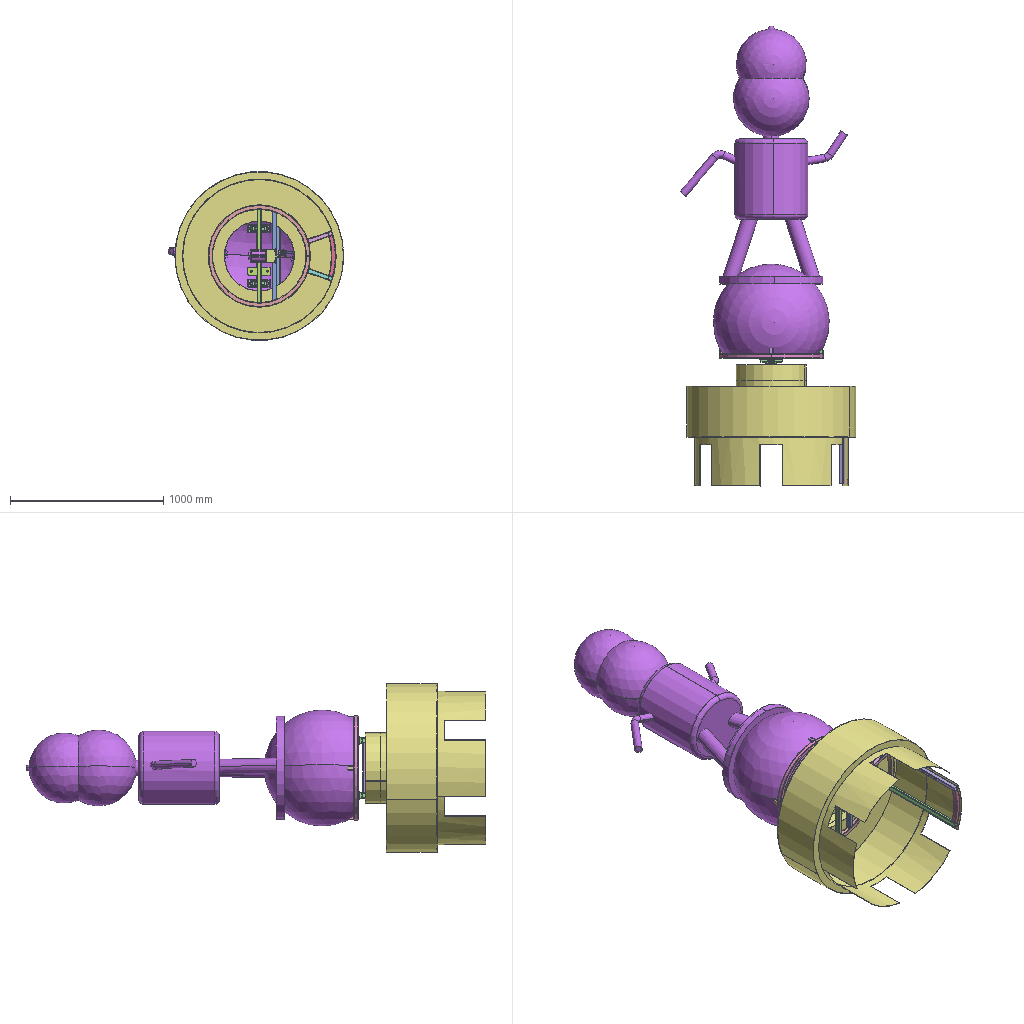Assembly | SolidWorks | 16 different items | 26 placed | box 1147 x 3005 x 1100 mm
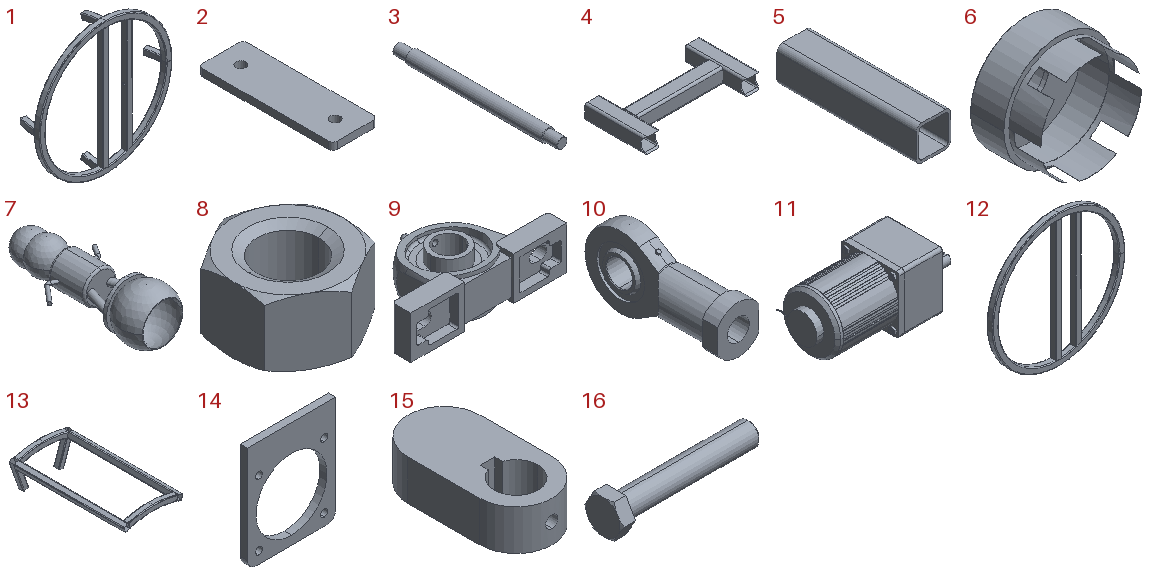Parts list (item | quantity | size | volume | features):
1 | x1 | 680 x 115 x 680 mm | 760065 mm3 | features ICE 3, WeldMemberFeat 2, CirPattern 1, WeldmentFeature 1
2 | x4 | 50 x 150 x 8 mm | 58308 mm3 | features Extrusion 1, HoleWzd 1
3 | x1 | 32 x 400 x 32 mm | 299686 mm3 | features Chamfer 1, Revolution 1
4 | x1 | 230 x 120 x 30 mm | 85383 mm3 | features ICE 1, WeldMemberFeat 1, WeldmentFeature 1
5 | x1 | 25 x 100 x 25 mm | 17370 mm3 | features WeldMemberFeat 1, WeldmentFeature 1
6 | x1 | 1104 x 790 x 1104 mm | 5979369 mm3 | features ICE 2, CirPattern 1, Revolution 1, Shell 1, WeldmentFeature 1
7 | x1 | 1093 x 2171 x 758 mm | 26788411 mm3 | features Sweep 4, ICE 3, Revolution 2, CombineBodies 1, Fillet 1, Shell 1
8 | x5 | 18 x 20.785 x 10.8 mm | 2109 mm3 | features ICE 2, RevCut 2, Extrusion 1
9 | x2 | 142 x 78.36 x 39.3 mm | 118845 mm3 | features Revolution 5, Cut 3, Boss 2, CirPattern 2, ICE 2, RevCut 2, Extrusion 1, RefAxis 1, SweepCut 1
10 | x1 | 19 x 67 x 34 mm | 14399 mm3 | features Revolution 3, ICE 2, RevCut 1
11 | x1 | 209 x 90.466 x 90 mm | 815406 mm3 | features ICE 12, Fillet 4, CirPattern 3, Chamfer 2, Revolution 2, Sweep 1
12 | x1 | 670 x 30 x 670 mm | 682937 mm3 | features ICE 1, WeldMemberFeat 1, WeldmentFeature 1
13 | x1 | 330 x 635 x 183.766 mm | 442860 mm3 | features 3DProfileFeature 1, WeldCornerFeat 1, WeldMemberFeat 1, WeldmentFeature 1
14 | x1 | 100 x 8 x 120 mm | 53836 mm3 | features CirPattern 1, Extrusion 1, Fillet 1, HoleWzd 1, ICE 1
15 | x1 | 25 x 50 x 14 mm | 12843 mm3 | features Extrusion 1, HoleWzd 1
16 | x3 | 77.5 x 20.785 x 18 mm | 9981 mm3 | features Chamfer 2, RevCut 2, Revolution 2, Extrusion 1, ICE 1
Mates (type | each side: item.copy, entity, surface, feature):
Width | 5.1 face plane Gb/t 6728—2002 Square hollow section steel 25×2-example.com(1) | 5.1 face plane Gb/t 6728—2002 Square hollow section steel 25×2-example.com(1) | 16.1 face plane Boss-Extrude1 | 16.1 face plane Boss-Extrude1
Concentric | 16.1 face cylinder Revolve1 | 8.1 face cylinder Boss-Extrude1
Coincident | 16.1 face plane Boss-Extrude1 | 8.1 face plane Boss-Extrude1
Concentric | 16.1 face cylinder Revolve1 | 10.1 face cylinder Cut-Revolve1
Parallel | 16.1 face plane Boss-Extrude1 | 10.1 face plane Cut-Extrude1
DistanceDim | 16.1 face plane Revolve1 | 10.1 face plane Revolve1
Coincident | 8.1 face plane Boss-Extrude1 | 10.1 face plane Revolve1
Coincident | 1.1 face plane Gb/t 6728—2002 Square hollow section steel 30×2-example.com(1) | 2.1 face plane Boss-Extrude1
DistanceDim | 16.2 face cylinder Revolve1 | 1.1 face plane Gb/t 6728—2002 Square hollow section steel 30×2-example.com(1)
Coincident | 1.1 face plane Gb/t 6728—2002 Square hollow section steel 30×2-example.com(1) | 16.2 face plane Boss-Extrude1
Coincident | 1.1 face plane Gb/t 6728—2002 Square hollow section steel 30×2-example.com(1) | 8.2 face plane Boss-Extrude1
Coincident | 2.1 face plane Boss-Extrude1 | 2.2 face plane Boss-Extrude1 | 2 times
Coincident | 2.1 face plane Boss-Extrude1 | 9.1 face plane Boss-Extrude1
Slot | 2.1 face cylinder Ø11.0 (11) Diameter Hole5 | 9.1 face cylinder Cut-Extrude3
Parallel | 2.1 face plane Boss-Extrude1 | 9.1 face plane Boss-Extrude1
DistanceDim | 2.2 face cylinder Ø11.0 (11) Diameter Hole5 | 2.1 face cylinder Ø11.0 (11) Diameter Hole5
Coincident | 2.2 face plane Boss-Extrude1 | 9.2 face plane Boss-Extrude1
Slot | 2.2 face cylinder Ø11.0 (11) Diameter Hole5 | 9.2 face cylinder Cut-Extrude3
Coincident | 2.3 face plane Boss-Extrude1 | 2.4 face plane Boss-Extrude1 | 3 times
Coincident | 4.1 face plane Gb/t 6728—2002 Square hollow section steel 30×2-example.com(1) | 2.3 face plane Boss-Extrude1
DistanceDim | 4.1 face plane Gb/t 6728—2002 Square hollow section steel 30×2-example.com(1) | 2.3 face plane Boss-Extrude1
Concentric | 3.1 face cylinder Revolve1 | 9.1 face cylinder Boss-Revolve5
Coincident | 3.1 face plane Revolve1 | 9.1 face plane Boss-Revolve5
Concentric | 3.1 face cylinder Revolve1 | 4.1 face cylinder Cut-Extrude1
Coincident | 9.1 face plane Boss-Extrude1 | 9.2 face plane Boss-Extrude1
Concentric | 8.2 face cylinder Boss-Extrude1 | 16.2 face cylinder Revolve1
DistanceDim | 8.3 face plane Boss-Extrude1 | 8.2 face plane Boss-Extrude1
Concentric | 16.2 face cylinder Revolve1 | 8.3 face cylinder Boss-Extrude1
Coincident | 1.1 face plane Gb/t 6728—2002 Square hollow section steel 30×2-example.com(1) | 7.1 face plane Revolve1
Concentric | 1.1 face cylinder Gb/t 6728—2002 Square hollow section steel 30×2-example.com(1) | 7.1 face cylinder Boss-Extrude2
Coincident | 11.1 face plane Boss-Extrude2 | 14.1 face plane Boss-Extrude1
Concentric | 11.1 face cylinder Cut-Extrude1 | 14.1 face cylinder Cut-Extrude1
Concentric | 11.1 face cylinder CirPattern3 | 14.1 face cylinder CirPattern1
Concentric | 11.1 face cylinder Revolve2 | 15.1 face cylinder Boss-Extrude1
Coincident | 11.1 face plane Revolve2 | 15.1 face plane Boss-Extrude1
Concentric | 15.1 face cylinder Boss-Extrude1 | 16.3 face cylinder Revolve1
Coincident | 15.1 face plane Boss-Extrude1 | 16.3 face plane Boss-Extrude1
Concentric | 16.3 face cylinder Revolve1 | 8.4 face cylinder Boss-Extrude1
Concentric | 16.3 face cylinder Revolve1 | 8.5 face cylinder Boss-Extrude1
Coincident | 8.4 face plane Boss-Extrude1 | 8.5 face plane Boss-Extrude1
Concentric | 16.3 face cylinder Revolve1 | 10.1 face cylinder Revolve2
Coincident | 8.4 face plane Boss-Extrude1 | 10.1 face plane Revolve2
Concentric | 12.1 face cylinder Gb/t 6728—2002 Square hollow section steel 30×2-example.com(1) | 13.1 face cylinder Gb/t 6728—2002 Square hollow section steel 30×2-example.com(1)
Coincident | 12.1 face plane Gb/t 6728—2002 Square hollow section steel 30×2-example.com(1) | 13.1 face plane Gb/t 6728—2002 Square hollow section steel 30×2-example.com(1)
Coincident | 12.1 face plane Gb/t 6728—2002 Square hollow section steel 30×2-example.com(1) | 6.1 face plane Shell1
Concentric | 12.1 face cylinder Gb/t 6728—2002 Square hollow section steel 30×2-example.com(1) | 1.1 face cylinder Gb/t 6728—2002 Square hollow section steel 30×2-example.com(1)
Parallel | 12.1 face plane Gb/t 6728—2002 Square hollow section steel 30×2-example.com(1) | 1.1 face plane Gb/t 6728—2002 Square hollow section steel 30×2-example.com(1)
Coincident | 12.1 face plane Gb/t 6728—2002 Square hollow section steel 30×2-example.com(1) | 14.1 face plane Boss-Extrude1 | 2 times